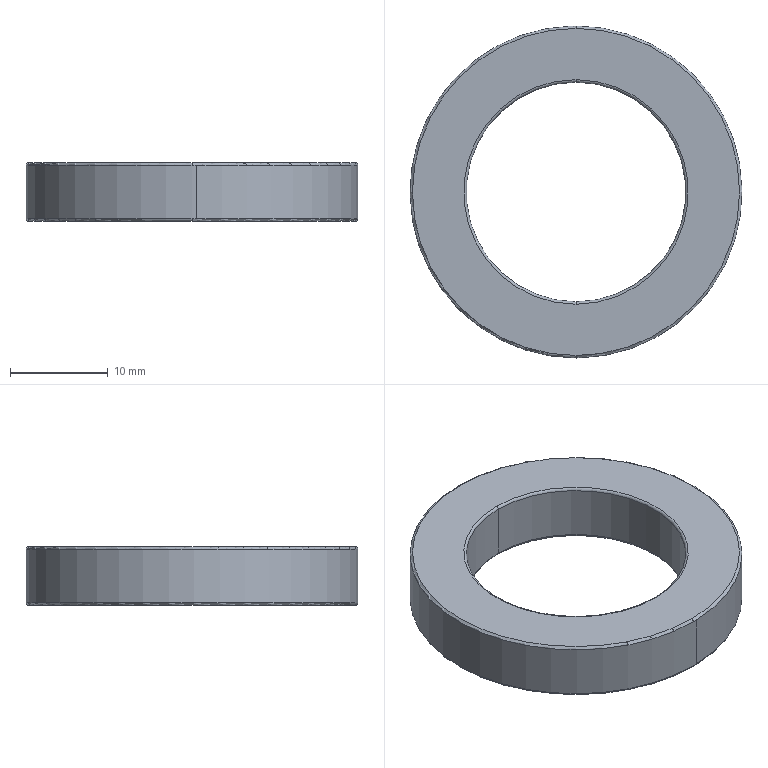Part | STEP file | 2026.6.15-Main Assembly图.sldasm-Part-116 | 1 solid | 14 faces | box 34 x 34 x 6 mm | volume 3057 mm3 | torus 8 | cylinder 4 | plane 2 | commonest cylinder face diameters 22.5 x2 34 x2
STEP:
#1=CARTESIAN_POINT('',(-1571.253,1407.256,3672.821));
#2=VERTEX_POINT('',#1);
#3=CARTESIAN_POINT('',(-1570.765,1407.263,3672.821));
#4=VERTEX_POINT('',#3);
#5=CARTESIAN_POINT('',(-1571.253,1424.256,3672.821));
#6=DIRECTION('',(0.,0.,1.));
#7=DIRECTION('',(0.,1.,0.));
#8=AXIS2_PLACEMENT_3D('',#5,#6,#7);
#9=CIRCLE('',#8,17.);
#10=EDGE_CURVE('',#2,#4,#9,.T.);
#11=ORIENTED_EDGE('',*,*,#10,.F.);
#12=CARTESIAN_POINT('',(-1571.253,1407.506,3672.571));
#13=VERTEX_POINT('',#12);
#14=CARTESIAN_POINT('',(-1571.253,1407.506,3672.821));
#15=DIRECTION('',(1.,0.,0.));
#16=DIRECTION('',(0.,0.,-1.));
#17=AXIS2_PLACEMENT_3D('',#14,#15,#16);
#18=CIRCLE('',#17,0.25);
#19=EDGE_CURVE('',#2,#13,#18,.T.);
#20=ORIENTED_EDGE('',*,*,#19,.T.);
#21=CARTESIAN_POINT('',(-1571.253,1441.006,3672.571));
#22=VERTEX_POINT('',#21);
#23=CARTESIAN_POINT('',(-1571.253,1424.256,3672.571));
#24=DIRECTION('',(0.,0.,-1.));
#25=DIRECTION('',(0.,1.,0.));
#26=AXIS2_PLACEMENT_3D('',#23,#24,#25);
#27=CIRCLE('',#26,16.75);
#28=EDGE_CURVE('',#22,#13,#27,.T.);
#29=ORIENTED_EDGE('',*,*,#28,.F.);
#30=CARTESIAN_POINT('',(-1571.253,1441.256,3672.821));
#31=VERTEX_POINT('',#30);
#32=CARTESIAN_POINT('',(-1571.253,1441.006,3672.821));
#33=DIRECTION('',(-1.,0.,0.));
#34=DIRECTION('',(0.,0.,1.));
#35=AXIS2_PLACEMENT_3D('',#32,#33,#34);
#36=CIRCLE('',#35,0.25);
#37=EDGE_CURVE('',#31,#22,#36,.T.);
#38=ORIENTED_EDGE('',*,*,#37,.F.);
#39=CARTESIAN_POINT('',(-1571.253,1424.256,3672.821));
#40=DIRECTION('',(0.,0.,1.));
#41=DIRECTION('',(0.,1.,0.));
#42=AXIS2_PLACEMENT_3D('',#39,#40,#41);
#43=CIRCLE('',#42,17.);
#44=EDGE_CURVE('',#4,#31,#43,.T.);
#45=ORIENTED_EDGE('',*,*,#44,.F.);
#46=EDGE_LOOP('',(#11,#20,#29,#38,#45));
#47=FACE_OUTER_BOUND('',#46,.T.);
#48=CARTESIAN_POINT('',(-1571.253,1424.256,3672.821));
#49=DIRECTION('',(0.,0.,-1.));
#50=DIRECTION('',(0.,1.,0.));
#51=AXIS2_PLACEMENT_3D('',#48,#49,#50);
#52=TOROIDAL_SURFACE('',#51,16.75,0.25);
#53=ADVANCED_FACE('',(#47),#52,.T.);
#54=CARTESIAN_POINT('',(-1571.253,1441.256,3678.321));
#55=VERTEX_POINT('',#54);
#56=CARTESIAN_POINT('',(-1570.765,1407.263,3678.321));
#57=VERTEX_POINT('',#56);
#58=CARTESIAN_POINT('',(-1571.253,1424.256,3678.321));
#59=DIRECTION('',(0.,0.,-1.));
#60=DIRECTION('',(0.,-1.,0.));
#61=AXIS2_PLACEMENT_3D('',#58,#59,#60);
#62=CIRCLE('',#61,17.);
#63=EDGE_CURVE('',#55,#57,#62,.T.);
#64=ORIENTED_EDGE('',*,*,#63,.F.);
#65=CARTESIAN_POINT('',(-1571.253,1441.006,3678.571));
#66=VERTEX_POINT('',#65);
#67=CARTESIAN_POINT('',(-1571.253,1441.006,3678.321));
#68=DIRECTION('',(1.,0.,0.));
#69=DIRECTION('',(0.,0.,-1.));
#70=AXIS2_PLACEMENT_3D('',#67,#68,#69);
#71=CIRCLE('',#70,0.25);
#72=EDGE_CURVE('',#55,#66,#71,.T.);
#73=ORIENTED_EDGE('',*,*,#72,.T.);
#74=CARTESIAN_POINT('',(-1571.253,1407.506,3678.571));
#75=VERTEX_POINT('',#74);
#76=CARTESIAN_POINT('',(-1571.253,1424.256,3678.571));
#77=DIRECTION('',(0.,0.,1.));
#78=DIRECTION('',(0.,-1.,0.));
#79=AXIS2_PLACEMENT_3D('',#76,#77,#78);
#80=CIRCLE('',#79,16.75);
#81=EDGE_CURVE('',#75,#66,#80,.T.);
#82=ORIENTED_EDGE('',*,*,#81,.F.);
#83=CARTESIAN_POINT('',(-1571.253,1407.256,3678.321));
#84=VERTEX_POINT('',#83);
#85=CARTESIAN_POINT('',(-1571.253,1407.506,3678.321));
#86=DIRECTION('',(-1.,0.,0.));
#87=DIRECTION('',(0.,0.,1.));
#88=AXIS2_PLACEMENT_3D('',#85,#86,#87);
#89=CIRCLE('',#88,0.25);
#90=EDGE_CURVE('',#84,#75,#89,.T.);
#91=ORIENTED_EDGE('',*,*,#90,.F.);
#92=CARTESIAN_POINT('',(-1571.253,1424.256,3678.321));
#93=DIRECTION('',(0.,0.,-1.));
#94=DIRECTION('',(0.,-1.,0.));
#95=AXIS2_PLACEMENT_3D('',#92,#93,#94);
#96=CIRCLE('',#95,17.);
#97=EDGE_CURVE('',#57,#84,#96,.T.);
#98=ORIENTED_EDGE('',*,*,#97,.F.);
#99=EDGE_LOOP('',(#64,#73,#82,#91,#98));
#100=FACE_OUTER_BOUND('',#99,.T.);
#101=CARTESIAN_POINT('',(-1571.253,1424.256,3678.321));
#102=DIRECTION('',(0.,0.,1.));
#103=DIRECTION('',(0.,-1.,0.));
#104=AXIS2_PLACEMENT_3D('',#101,#102,#103);
#105=TOROIDAL_SURFACE('',#104,16.75,0.25);
#106=ADVANCED_FACE('',(#100),#105,.T.);
#107=CARTESIAN_POINT('',(-1571.253,1412.756,3672.571));
#108=VERTEX_POINT('',#107);
#109=CARTESIAN_POINT('',(-1571.253,1435.756,3672.571));
#110=VERTEX_POINT('',#109);
#111=CARTESIAN_POINT('',(-1571.253,1424.256,3672.571));
#112=DIRECTION('',(0.,0.,1.));
#113=DIRECTION('',(0.,1.,0.));
#114=AXIS2_PLACEMENT_3D('',#111,#112,#113);
#115=CIRCLE('',#114,11.5);
#116=EDGE_CURVE('',#108,#110,#115,.T.);
#117=ORIENTED_EDGE('',*,*,#116,.F.);
#118=CARTESIAN_POINT('',(-1571.253,1413.006,3672.821));
#119=VERTEX_POINT('',#118);
#120=CARTESIAN_POINT('',(-1571.253,1412.756,3672.821));
#121=DIRECTION('',(1.,0.,0.));
#122=DIRECTION('',(0.,0.,-1.));
#123=AXIS2_PLACEMENT_3D('',#120,#121,#122);
#124=CIRCLE('',#123,0.25);
#125=EDGE_CURVE('',#108,#119,#124,.T.);
#126=ORIENTED_EDGE('',*,*,#125,.T.);
#127=CARTESIAN_POINT('',(-1571.253,1435.506,3672.821));
#128=VERTEX_POINT('',#127);
#129=CARTESIAN_POINT('',(-1571.253,1424.256,3672.821));
#130=DIRECTION('',(0.,0.,-1.));
#131=DIRECTION('',(0.,1.,0.));
#132=AXIS2_PLACEMENT_3D('',#129,#130,#131);
#133=CIRCLE('',#132,11.25);
#134=EDGE_CURVE('',#128,#119,#133,.T.);
#135=ORIENTED_EDGE('',*,*,#134,.F.);
#136=CARTESIAN_POINT('',(-1571.253,1435.756,3672.821));
#137=DIRECTION('',(-1.,0.,0.));
#138=DIRECTION('',(0.,0.,1.));
#139=AXIS2_PLACEMENT_3D('',#136,#137,#138);
#140=CIRCLE('',#139,0.25);
#141=EDGE_CURVE('',#110,#128,#140,.T.);
#142=ORIENTED_EDGE('',*,*,#141,.F.);
#143=EDGE_LOOP('',(#117,#126,#135,#142));
#144=FACE_OUTER_BOUND('',#143,.T.);
#145=CARTESIAN_POINT('',(-1571.253,1424.256,3672.821));
#146=DIRECTION('',(0.,0.,-1.));
#147=DIRECTION('',(0.,1.,0.));
#148=AXIS2_PLACEMENT_3D('',#145,#146,#147);
#149=TOROIDAL_SURFACE('',#148,11.5,0.25);
#150=ADVANCED_FACE('',(#144),#149,.T.);
#151=CARTESIAN_POINT('',(-1571.253,1435.756,3678.571));
#152=VERTEX_POINT('',#151);
#153=CARTESIAN_POINT('',(-1571.253,1412.756,3678.571));
#154=VERTEX_POINT('',#153);
#155=CARTESIAN_POINT('',(-1571.253,1424.256,3678.571));
#156=DIRECTION('',(0.,0.,-1.));
#157=DIRECTION('',(0.,-1.,0.));
#158=AXIS2_PLACEMENT_3D('',#155,#156,#157);
#159=CIRCLE('',#158,11.5);
#160=EDGE_CURVE('',#152,#154,#159,.T.);
#161=ORIENTED_EDGE('',*,*,#160,.F.);
#162=CARTESIAN_POINT('',(-1571.253,1435.506,3678.321));
#163=VERTEX_POINT('',#162);
#164=CARTESIAN_POINT('',(-1571.253,1435.756,3678.321));
#165=DIRECTION('',(1.,0.,0.));
#166=DIRECTION('',(0.,0.,-1.));
#167=AXIS2_PLACEMENT_3D('',#164,#165,#166);
#168=CIRCLE('',#167,0.25);
#169=EDGE_CURVE('',#152,#163,#168,.T.);
#170=ORIENTED_EDGE('',*,*,#169,.T.);
#171=CARTESIAN_POINT('',(-1571.253,1413.006,3678.321));
#172=VERTEX_POINT('',#171);
#173=CARTESIAN_POINT('',(-1571.253,1424.256,3678.321));
#174=DIRECTION('',(0.,0.,1.));
#175=DIRECTION('',(0.,-1.,0.));
#176=AXIS2_PLACEMENT_3D('',#173,#174,#175);
#177=CIRCLE('',#176,11.25);
#178=EDGE_CURVE('',#172,#163,#177,.T.);
#179=ORIENTED_EDGE('',*,*,#178,.F.);
#180=CARTESIAN_POINT('',(-1571.253,1412.756,3678.321));
#181=DIRECTION('',(-1.,0.,0.));
#182=DIRECTION('',(0.,0.,1.));
#183=AXIS2_PLACEMENT_3D('',#180,#181,#182);
#184=CIRCLE('',#183,0.25);
#185=EDGE_CURVE('',#154,#172,#184,.T.);
#186=ORIENTED_EDGE('',*,*,#185,.F.);
#187=EDGE_LOOP('',(#161,#170,#179,#186));
#188=FACE_OUTER_BOUND('',#187,.T.);
#189=CARTESIAN_POINT('',(-1571.253,1424.256,3678.321));
#190=DIRECTION('',(0.,0.,1.));
#191=DIRECTION('',(0.,-1.,0.));
#192=AXIS2_PLACEMENT_3D('',#189,#190,#191);
#193=TOROIDAL_SURFACE('',#192,11.5,0.25);
#194=ADVANCED_FACE('',(#188),#193,.T.);
#195=CARTESIAN_POINT('',(-1571.253,1424.256,3678.321));
#196=DIRECTION('',(0.,0.,1.));
#197=DIRECTION('',(0.,-1.,0.));
#198=AXIS2_PLACEMENT_3D('',#195,#196,#197);
#199=CIRCLE('',#198,11.25);
#200=EDGE_CURVE('',#163,#172,#199,.T.);
#201=ORIENTED_EDGE('',*,*,#200,.T.);
#202=CARTESIAN_POINT('',(-1571.253,1413.006,3678.571));
#203=DIRECTION('',(0.,0.,-1.));
#204=VECTOR('',#203,1000.);
#205=LINE('',#202,#204);
#206=EDGE_CURVE('',#172,#119,#205,.T.);
#207=ORIENTED_EDGE('',*,*,#206,.T.);
#208=CARTESIAN_POINT('',(-1571.253,1424.256,3672.821));
#209=DIRECTION('',(0.,0.,-1.));
#210=DIRECTION('',(0.,1.,0.));
#211=AXIS2_PLACEMENT_3D('',#208,#209,#210);
#212=CIRCLE('',#211,11.25);
#213=EDGE_CURVE('',#119,#128,#212,.T.);
#214=ORIENTED_EDGE('',*,*,#213,.T.);
#215=CARTESIAN_POINT('',(-1571.253,1435.506,3678.571));
#216=DIRECTION('',(0.,0.,-1.));
#217=VECTOR('',#216,1000.);
#218=LINE('',#215,#217);
#219=EDGE_CURVE('',#163,#128,#218,.T.);
#220=ORIENTED_EDGE('',*,*,#219,.F.);
#221=EDGE_LOOP('',(#201,#207,#214,#220));
#222=FACE_OUTER_BOUND('',#221,.T.);
#223=CARTESIAN_POINT('',(-1571.253,1424.256,3678.571));
#224=DIRECTION('',(0.,0.,-1.));
#225=DIRECTION('',(0.,1.,0.));
#226=AXIS2_PLACEMENT_3D('',#223,#224,#225);
#227=CYLINDRICAL_SURFACE('',#226,11.25);
#228=ADVANCED_FACE('',(#222),#227,.F.);
#229=ORIENTED_EDGE('',*,*,#97,.T.);
#230=CARTESIAN_POINT('',(-1571.741,1441.249,3678.321));
#231=VERTEX_POINT('',#230);
#232=CARTESIAN_POINT('',(-1571.253,1424.256,3678.321));
#233=DIRECTION('',(0.,0.,-1.));
#234=DIRECTION('',(0.,-1.,0.));
#235=AXIS2_PLACEMENT_3D('',#232,#233,#234);
#236=CIRCLE('',#235,17.);
#237=EDGE_CURVE('',#84,#231,#236,.T.);
#238=ORIENTED_EDGE('',*,*,#237,.T.);
#239=CARTESIAN_POINT('',(-1571.741,1441.249,3672.821));
#240=VERTEX_POINT('',#239);
#241=CARTESIAN_POINT('',(-1571.741,1441.249,3678.571));
#242=DIRECTION('',(0.,0.,-1.));
#243=VECTOR('',#242,1000.);
#244=LINE('',#241,#243);
#245=EDGE_CURVE('',#231,#240,#244,.T.);
#246=ORIENTED_EDGE('',*,*,#245,.T.);
#247=CARTESIAN_POINT('',(-1571.253,1424.256,3672.821));
#248=DIRECTION('',(0.,0.,1.));
#249=DIRECTION('',(0.,1.,0.));
#250=AXIS2_PLACEMENT_3D('',#247,#248,#249);
#251=CIRCLE('',#250,17.);
#252=EDGE_CURVE('',#240,#2,#251,.T.);
#253=ORIENTED_EDGE('',*,*,#252,.T.);
#254=ORIENTED_EDGE('',*,*,#10,.T.);
#255=CARTESIAN_POINT('',(-1570.765,1407.263,3678.571));
#256=DIRECTION('',(0.,0.,-1.));
#257=VECTOR('',#256,1000.);
#258=LINE('',#255,#257);
#259=EDGE_CURVE('',#57,#4,#258,.T.);
#260=ORIENTED_EDGE('',*,*,#259,.F.);
#261=EDGE_LOOP('',(#229,#238,#246,#253,#254,#260));
#262=FACE_OUTER_BOUND('',#261,.T.);
#263=CARTESIAN_POINT('',(-1571.253,1424.256,3678.571));
#264=DIRECTION('',(0.,0.,-1.));
#265=DIRECTION('',(0.02871,-0.9996,0.));
#266=AXIS2_PLACEMENT_3D('',#263,#264,#265);
#267=CYLINDRICAL_SURFACE('',#266,17.);
#268=ADVANCED_FACE('',(#262),#267,.T.);
#269=CARTESIAN_POINT('',(-1571.253,1424.256,3672.571));
#270=DIRECTION('',(0.,0.,1.));
#271=DIRECTION('',(0.,1.,0.));
#272=AXIS2_PLACEMENT_3D('',#269,#270,#271);
#273=CIRCLE('',#272,11.5);
#274=EDGE_CURVE('',#110,#108,#273,.T.);
#275=ORIENTED_EDGE('',*,*,#274,.T.);
#276=ORIENTED_EDGE('',*,*,#116,.T.);
#277=EDGE_LOOP('',(#275,#276));
#278=FACE_BOUND('',#277,.T.);
#279=ORIENTED_EDGE('',*,*,#28,.T.);
#280=CARTESIAN_POINT('',(-1571.253,1424.256,3672.571));
#281=DIRECTION('',(0.,0.,-1.));
#282=DIRECTION('',(0.,1.,0.));
#283=AXIS2_PLACEMENT_3D('',#280,#281,#282);
#284=CIRCLE('',#283,16.75);
#285=EDGE_CURVE('',#13,#22,#284,.T.);
#286=ORIENTED_EDGE('',*,*,#285,.T.);
#287=EDGE_LOOP('',(#279,#286));
#288=FACE_OUTER_BOUND('',#287,.T.);
#289=CARTESIAN_POINT('',(-1571.253,1424.256,3672.571));
#290=DIRECTION('',(0.,0.,-1.));
#291=DIRECTION('',(0.,1.,0.));
#292=AXIS2_PLACEMENT_3D('',#289,#290,#291);
#293=PLANE('',#292);
#294=ADVANCED_FACE('',(#278,#288),#293,.T.);
#295=CARTESIAN_POINT('',(-1571.253,1424.256,3678.571));
#296=DIRECTION('',(0.,0.,-1.));
#297=DIRECTION('',(0.,-1.,0.));
#298=AXIS2_PLACEMENT_3D('',#295,#296,#297);
#299=CIRCLE('',#298,11.5);
#300=EDGE_CURVE('',#154,#152,#299,.T.);
#301=ORIENTED_EDGE('',*,*,#300,.T.);
#302=ORIENTED_EDGE('',*,*,#160,.T.);
#303=EDGE_LOOP('',(#301,#302));
#304=FACE_BOUND('',#303,.T.);
#305=ORIENTED_EDGE('',*,*,#81,.T.);
#306=CARTESIAN_POINT('',(-1571.253,1424.256,3678.571));
#307=DIRECTION('',(0.,0.,1.));
#308=DIRECTION('',(0.,-1.,0.));
#309=AXIS2_PLACEMENT_3D('',#306,#307,#308);
#310=CIRCLE('',#309,16.75);
#311=EDGE_CURVE('',#66,#75,#310,.T.);
#312=ORIENTED_EDGE('',*,*,#311,.T.);
#313=EDGE_LOOP('',(#305,#312));
#314=FACE_OUTER_BOUND('',#313,.T.);
#315=CARTESIAN_POINT('',(-1571.253,1424.256,3678.571));
#316=DIRECTION('',(0.,0.,1.));
#317=DIRECTION('',(0.,-1.,0.));
#318=AXIS2_PLACEMENT_3D('',#315,#316,#317);
#319=PLANE('',#318);
#320=ADVANCED_FACE('',(#304,#314),#319,.T.);
#321=ORIENTED_EDGE('',*,*,#245,.F.);
#322=CARTESIAN_POINT('',(-1571.253,1424.256,3678.321));
#323=DIRECTION('',(0.,0.,-1.));
#324=DIRECTION('',(0.,-1.,0.));
#325=AXIS2_PLACEMENT_3D('',#322,#323,#324);
#326=CIRCLE('',#325,17.);
#327=EDGE_CURVE('',#231,#55,#326,.T.);
#328=ORIENTED_EDGE('',*,*,#327,.T.);
#329=ORIENTED_EDGE('',*,*,#63,.T.);
#330=ORIENTED_EDGE('',*,*,#259,.T.);
#331=ORIENTED_EDGE('',*,*,#44,.T.);
#332=CARTESIAN_POINT('',(-1571.253,1424.256,3672.821));
#333=DIRECTION('',(0.,0.,1.));
#334=DIRECTION('',(0.,1.,0.));
#335=AXIS2_PLACEMENT_3D('',#332,#333,#334);
#336=CIRCLE('',#335,17.);
#337=EDGE_CURVE('',#31,#240,#336,.T.);
#338=ORIENTED_EDGE('',*,*,#337,.T.);
#339=EDGE_LOOP('',(#321,#328,#329,#330,#331,#338));
#340=FACE_OUTER_BOUND('',#339,.T.);
#341=CARTESIAN_POINT('',(-1571.253,1424.256,3678.571));
#342=DIRECTION('',(0.,0.,-1.));
#343=DIRECTION('',(0.02871,-0.9996,0.));
#344=AXIS2_PLACEMENT_3D('',#341,#342,#343);
#345=CYLINDRICAL_SURFACE('',#344,17.);
#346=ADVANCED_FACE('',(#340),#345,.T.);
#347=ORIENTED_EDGE('',*,*,#206,.F.);
#348=ORIENTED_EDGE('',*,*,#178,.T.);
#349=ORIENTED_EDGE('',*,*,#219,.T.);
#350=ORIENTED_EDGE('',*,*,#134,.T.);
#351=EDGE_LOOP('',(#347,#348,#349,#350));
#352=FACE_OUTER_BOUND('',#351,.T.);
#353=CARTESIAN_POINT('',(-1571.253,1424.256,3678.571));
#354=DIRECTION('',(0.,0.,-1.));
#355=DIRECTION('',(0.,1.,0.));
#356=AXIS2_PLACEMENT_3D('',#353,#354,#355);
#357=CYLINDRICAL_SURFACE('',#356,11.25);
#358=ADVANCED_FACE('',(#352),#357,.F.);
#359=ORIENTED_EDGE('',*,*,#169,.F.);
#360=ORIENTED_EDGE('',*,*,#300,.F.);
#361=ORIENTED_EDGE('',*,*,#185,.T.);
#362=ORIENTED_EDGE('',*,*,#200,.F.);
#363=EDGE_LOOP('',(#359,#360,#361,#362));
#364=FACE_OUTER_BOUND('',#363,.T.);
#365=CARTESIAN_POINT('',(-1571.253,1424.256,3678.321));
#366=DIRECTION('',(0.,0.,1.));
#367=DIRECTION('',(0.,-1.,0.));
#368=AXIS2_PLACEMENT_3D('',#365,#366,#367);
#369=TOROIDAL_SURFACE('',#368,11.5,0.25);
#370=ADVANCED_FACE('',(#364),#369,.T.);
#371=ORIENTED_EDGE('',*,*,#125,.F.);
#372=ORIENTED_EDGE('',*,*,#274,.F.);
#373=ORIENTED_EDGE('',*,*,#141,.T.);
#374=ORIENTED_EDGE('',*,*,#213,.F.);
#375=EDGE_LOOP('',(#371,#372,#373,#374));
#376=FACE_OUTER_BOUND('',#375,.T.);
#377=CARTESIAN_POINT('',(-1571.253,1424.256,3672.821));
#378=DIRECTION('',(0.,0.,-1.));
#379=DIRECTION('',(0.,1.,0.));
#380=AXIS2_PLACEMENT_3D('',#377,#378,#379);
#381=TOROIDAL_SURFACE('',#380,11.5,0.25);
#382=ADVANCED_FACE('',(#376),#381,.T.);
#383=ORIENTED_EDGE('',*,*,#72,.F.);
#384=ORIENTED_EDGE('',*,*,#327,.F.);
#385=ORIENTED_EDGE('',*,*,#237,.F.);
#386=ORIENTED_EDGE('',*,*,#90,.T.);
#387=ORIENTED_EDGE('',*,*,#311,.F.);
#388=EDGE_LOOP('',(#383,#384,#385,#386,#387));
#389=FACE_OUTER_BOUND('',#388,.T.);
#390=CARTESIAN_POINT('',(-1571.253,1424.256,3678.321));
#391=DIRECTION('',(0.,0.,1.));
#392=DIRECTION('',(0.,-1.,0.));
#393=AXIS2_PLACEMENT_3D('',#390,#391,#392);
#394=TOROIDAL_SURFACE('',#393,16.75,0.25);
#395=ADVANCED_FACE('',(#389),#394,.T.);
#396=ORIENTED_EDGE('',*,*,#19,.F.);
#397=ORIENTED_EDGE('',*,*,#252,.F.);
#398=ORIENTED_EDGE('',*,*,#337,.F.);
#399=ORIENTED_EDGE('',*,*,#37,.T.);
#400=ORIENTED_EDGE('',*,*,#285,.F.);
#401=EDGE_LOOP('',(#396,#397,#398,#399,#400));
#402=FACE_OUTER_BOUND('',#401,.T.);
#403=CARTESIAN_POINT('',(-1571.253,1424.256,3672.821));
#404=DIRECTION('',(0.,0.,-1.));
#405=DIRECTION('',(0.,1.,0.));
#406=AXIS2_PLACEMENT_3D('',#403,#404,#405);
#407=TOROIDAL_SURFACE('',#406,16.75,0.25);
#408=ADVANCED_FACE('',(#402),#407,.T.);
#409=CLOSED_SHELL('',(#53,#106,#150,#194,#228,#268,#294,#320,#346,#358,#370,#382,#395,#408));
#410=MANIFOLD_SOLID_BREP('',#409);
#411=CARTESIAN_POINT('',(0.,0.,0.));
#412=DIRECTION('',(0.,0.,1.));
#413=DIRECTION('',(1.,0.,0.));
#414=AXIS2_PLACEMENT_3D('',#411,#412,#413);
#415=(LENGTH_UNIT()NAMED_UNIT(*)SI_UNIT(.MILLI.,.METRE.));
#416=UNCERTAINTY_MEASURE_WITH_UNIT(LENGTH_MEASURE(0.00001),#415,'','');
#417=(NAMED_UNIT(*)PLANE_ANGLE_UNIT()SI_UNIT($,.RADIAN.));
#418=(NAMED_UNIT(*)SI_UNIT($,.STERADIAN.)SOLID_ANGLE_UNIT());
#419=(GEOMETRIC_REPRESENTATION_CONTEXT(3)GLOBAL_UNCERTAINTY_ASSIGNED_CONTEXT((#416))GLOBAL_UNIT_ASSIGNED_CONTEXT((#415,#417,#418))REPRESENTATION_CONTEXT('',''));
#420=ADVANCED_BREP_SHAPE_REPRESENTATION('',(#410,#414),#419);